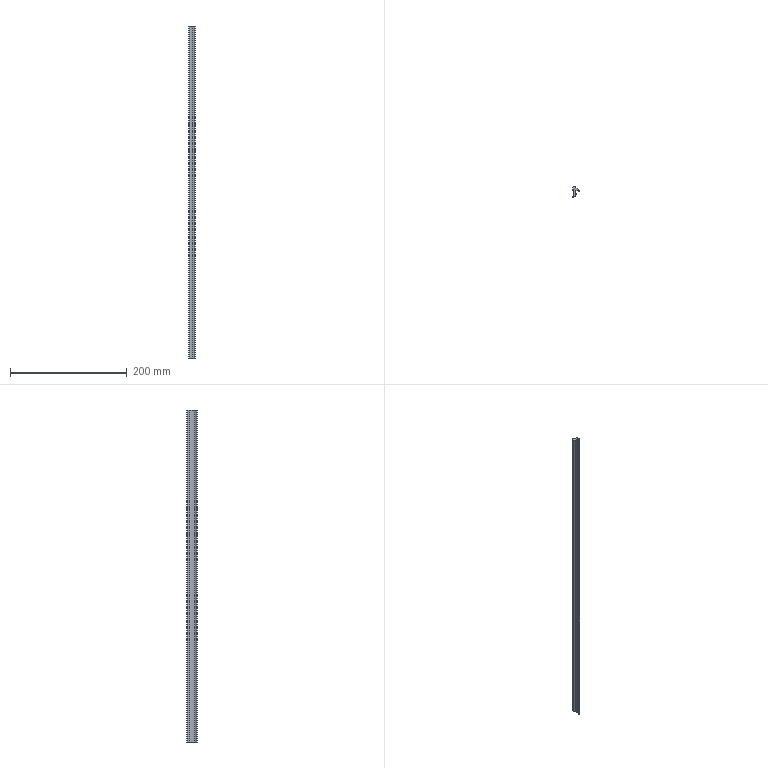Part | SolidWorks | features BaseBody 1, MoveFace 1 | 1 solid | 20 faces | box 10.8 x 17.5 x 568 mm | volume 44759 mm3 | cylinder 11 | plane 9 | commonest cylinder face diameters 1.6 x2 14 x2 0.4 x1 0.6 x1 0.8 x1 2.6 x1
STEP:
#1=CARTESIAN_POINT('',(-3.236,-11.055,468.));
#2=VERTEX_POINT('',#1);
#3=CARTESIAN_POINT('',(-4.3,-10.3,468.));
#4=VERTEX_POINT('',#3);
#5=CARTESIAN_POINT('',(-3.5,-10.3,468.));
#6=DIRECTION('',(0.,0.,-1.));
#7=DIRECTION('',(1.,0.,0.));
#8=AXIS2_PLACEMENT_3D('',#5,#6,#7);
#9=CIRCLE('',#8,0.8);
#10=EDGE_CURVE('',#2,#4,#9,.T.);
#11=ORIENTED_EDGE('',*,*,#10,.T.);
#12=CARTESIAN_POINT('',(-4.3,-10.3,-100.));
#13=VERTEX_POINT('',#12);
#14=CARTESIAN_POINT('',(-4.3,-10.3,-100.));
#15=DIRECTION('',(0.,0.,-1.));
#16=VECTOR('',#15,1000.);
#17=LINE('',#14,#16);
#18=EDGE_CURVE('',#4,#13,#17,.T.);
#19=ORIENTED_EDGE('',*,*,#18,.T.);
#20=CARTESIAN_POINT('',(-3.236,-11.055,-100.));
#21=VERTEX_POINT('',#20);
#22=CARTESIAN_POINT('',(-3.5,-10.3,-100.));
#23=DIRECTION('',(0.,0.,1.));
#24=DIRECTION('',(-1.,0.,0.));
#25=AXIS2_PLACEMENT_3D('',#22,#23,#24);
#26=CIRCLE('',#25,0.8);
#27=EDGE_CURVE('',#13,#21,#26,.T.);
#28=ORIENTED_EDGE('',*,*,#27,.T.);
#29=CARTESIAN_POINT('',(-3.236,-11.055,-100.));
#30=DIRECTION('',(0.,0.,-1.));
#31=VECTOR('',#30,1000.);
#32=LINE('',#29,#31);
#33=EDGE_CURVE('',#2,#21,#32,.T.);
#34=ORIENTED_EDGE('',*,*,#33,.F.);
#35=EDGE_LOOP('',(#11,#19,#28,#34));
#36=FACE_OUTER_BOUND('',#35,.T.);
#37=CARTESIAN_POINT('',(-3.5,-10.3,-100.));
#38=DIRECTION('',(0.,0.,-1.));
#39=DIRECTION('',(-1.,0.,0.));
#40=AXIS2_PLACEMENT_3D('',#37,#38,#39);
#41=CYLINDRICAL_SURFACE('',#40,0.8);
#42=ADVANCED_FACE('',(#36),#41,.T.);
#43=CARTESIAN_POINT('',(1.184,-6.397,-100.));
#44=VERTEX_POINT('',#43);
#45=CARTESIAN_POINT('',(-5.702,-4.29,-100.));
#46=DIRECTION('',(0.,0.,1.));
#47=DIRECTION('',(-1.,0.,0.));
#48=AXIS2_PLACEMENT_3D('',#45,#46,#47);
#49=CIRCLE('',#48,7.201);
#50=EDGE_CURVE('',#21,#44,#49,.T.);
#51=ORIENTED_EDGE('',*,*,#50,.T.);
#52=CARTESIAN_POINT('',(1.184,-6.397,468.));
#53=VERTEX_POINT('',#52);
#54=CARTESIAN_POINT('',(1.184,-6.397,-100.));
#55=DIRECTION('',(0.,0.,1.));
#56=VECTOR('',#55,1000.);
#57=LINE('',#54,#56);
#58=EDGE_CURVE('',#44,#53,#57,.T.);
#59=ORIENTED_EDGE('',*,*,#58,.T.);
#60=CARTESIAN_POINT('',(-5.702,-4.29,468.));
#61=DIRECTION('',(0.,0.,-1.));
#62=DIRECTION('',(1.,0.,0.));
#63=AXIS2_PLACEMENT_3D('',#60,#61,#62);
#64=CIRCLE('',#63,7.201);
#65=EDGE_CURVE('',#53,#2,#64,.T.);
#66=ORIENTED_EDGE('',*,*,#65,.T.);
#67=ORIENTED_EDGE('',*,*,#33,.T.);
#68=EDGE_LOOP('',(#51,#59,#66,#67));
#69=FACE_OUTER_BOUND('',#68,.T.);
#70=CARTESIAN_POINT('',(-5.702,-4.29,-100.));
#71=DIRECTION('',(0.,0.,-1.));
#72=DIRECTION('',(-1.,0.,0.));
#73=AXIS2_PLACEMENT_3D('',#70,#71,#72);
#74=CYLINDRICAL_SURFACE('',#73,7.201);
#75=ADVANCED_FACE('',(#69),#74,.T.);
#76=CARTESIAN_POINT('',(0.9,-6.,-100.));
#77=VERTEX_POINT('',#76);
#78=CARTESIAN_POINT('',(0.9,-6.3,-100.));
#79=DIRECTION('',(0.,0.,1.));
#80=DIRECTION('',(-1.,0.,0.));
#81=AXIS2_PLACEMENT_3D('',#78,#79,#80);
#82=CIRCLE('',#81,0.3);
#83=EDGE_CURVE('',#44,#77,#82,.T.);
#84=ORIENTED_EDGE('',*,*,#83,.T.);
#85=CARTESIAN_POINT('',(0.9,-6.,468.));
#86=VERTEX_POINT('',#85);
#87=CARTESIAN_POINT('',(0.9,-6.,-100.));
#88=DIRECTION('',(0.,0.,1.));
#89=VECTOR('',#88,1000.);
#90=LINE('',#87,#89);
#91=EDGE_CURVE('',#77,#86,#90,.T.);
#92=ORIENTED_EDGE('',*,*,#91,.T.);
#93=CARTESIAN_POINT('',(0.9,-6.3,468.));
#94=DIRECTION('',(0.,0.,-1.));
#95=DIRECTION('',(1.,0.,0.));
#96=AXIS2_PLACEMENT_3D('',#93,#94,#95);
#97=CIRCLE('',#96,0.3);
#98=EDGE_CURVE('',#86,#53,#97,.T.);
#99=ORIENTED_EDGE('',*,*,#98,.T.);
#100=ORIENTED_EDGE('',*,*,#58,.F.);
#101=EDGE_LOOP('',(#84,#92,#99,#100));
#102=FACE_OUTER_BOUND('',#101,.T.);
#103=CARTESIAN_POINT('',(0.9,-6.3,-100.));
#104=DIRECTION('',(0.,0.,-1.));
#105=DIRECTION('',(-1.,0.,0.));
#106=AXIS2_PLACEMENT_3D('',#103,#104,#105);
#107=CYLINDRICAL_SURFACE('',#106,0.3);
#108=ADVANCED_FACE('',(#102),#107,.T.);
#109=CARTESIAN_POINT('',(-2.5,-0.5,-100.));
#110=VERTEX_POINT('',#109);
#111=CARTESIAN_POINT('',(-2.5,-6.153,-100.));
#112=VERTEX_POINT('',#111);
#113=CARTESIAN_POINT('',(-2.5,-6.397,-100.));
#114=DIRECTION('',(0.,-1.,0.));
#115=VECTOR('',#114,1000.);
#116=LINE('',#113,#115);
#117=EDGE_CURVE('',#110,#112,#116,.T.);
#118=ORIENTED_EDGE('',*,*,#117,.F.);
#119=CARTESIAN_POINT('',(-4.2,1.695,-100.));
#120=VERTEX_POINT('',#119);
#121=CARTESIAN_POINT('',(-1.701,1.875,-100.));
#122=DIRECTION('',(0.,0.,1.));
#123=DIRECTION('',(-1.,0.,0.));
#124=AXIS2_PLACEMENT_3D('',#121,#122,#123);
#125=CIRCLE('',#124,2.506);
#126=EDGE_CURVE('',#120,#110,#125,.T.);
#127=ORIENTED_EDGE('',*,*,#126,.F.);
#128=CARTESIAN_POINT('',(-4.2,5.1,-100.));
#129=VERTEX_POINT('',#128);
#130=CARTESIAN_POINT('',(-4.2,-6.397,-100.));
#131=DIRECTION('',(0.,-1.,0.));
#132=VECTOR('',#131,1000.);
#133=LINE('',#130,#132);
#134=EDGE_CURVE('',#129,#120,#133,.T.);
#135=ORIENTED_EDGE('',*,*,#134,.F.);
#136=CARTESIAN_POINT('',(-2.892,6.4,-100.));
#137=VERTEX_POINT('',#136);
#138=CARTESIAN_POINT('',(-2.9,5.1,-100.));
#139=DIRECTION('',(0.,0.,1.));
#140=DIRECTION('',(-1.,0.,0.));
#141=AXIS2_PLACEMENT_3D('',#138,#139,#140);
#142=CIRCLE('',#141,1.3);
#143=EDGE_CURVE('',#137,#129,#142,.T.);
#144=ORIENTED_EDGE('',*,*,#143,.F.);
#145=CARTESIAN_POINT('',(0.5,5.5,-100.));
#146=VERTEX_POINT('',#145);
#147=CARTESIAN_POINT('',(-2.934,-0.5999,-100.));
#148=DIRECTION('',(0.,0.,1.));
#149=DIRECTION('',(-1.,0.,0.));
#150=AXIS2_PLACEMENT_3D('',#147,#148,#149);
#151=CIRCLE('',#150,7.);
#152=EDGE_CURVE('',#146,#137,#151,.T.);
#153=ORIENTED_EDGE('',*,*,#152,.F.);
#154=CARTESIAN_POINT('',(5.5,1.7,-100.));
#155=VERTEX_POINT('',#154);
#156=CARTESIAN_POINT('',(5.5,1.7,-100.));
#157=DIRECTION('',(-0.7962,0.6051,0.));
#158=VECTOR('',#157,1000.);
#159=LINE('',#156,#158);
#160=EDGE_CURVE('',#155,#146,#159,.T.);
#161=ORIENTED_EDGE('',*,*,#160,.F.);
#162=CARTESIAN_POINT('',(6.458,-0.2215,-100.));
#163=VERTEX_POINT('',#162);
#164=CARTESIAN_POINT('',(6.458,-0.2215,-100.));
#165=DIRECTION('',(-0.4462,0.8949,0.));
#166=VECTOR('',#165,1000.);
#167=LINE('',#164,#166);
#168=EDGE_CURVE('',#163,#155,#167,.T.);
#169=ORIENTED_EDGE('',*,*,#168,.F.);
#170=CARTESIAN_POINT('',(5.895,-0.7433,-100.));
#171=VERTEX_POINT('',#170);
#172=CARTESIAN_POINT('',(6.1,-0.4,-100.));
#173=DIRECTION('',(0.,0.,1.));
#174=DIRECTION('',(-1.,0.,0.));
#175=AXIS2_PLACEMENT_3D('',#172,#173,#174);
#176=CIRCLE('',#175,0.4);
#177=EDGE_CURVE('',#171,#163,#176,.T.);
#178=ORIENTED_EDGE('',*,*,#177,.F.);
#179=CARTESIAN_POINT('',(3.,0.,-100.));
#180=VERTEX_POINT('',#179);
#181=CARTESIAN_POINT('',(2.746,-6.995,-100.));
#182=DIRECTION('',(0.,0.,-1.));
#183=DIRECTION('',(-1.,0.,0.));
#184=AXIS2_PLACEMENT_3D('',#181,#182,#183);
#185=CIRCLE('',#184,7.);
#186=EDGE_CURVE('',#180,#171,#185,.T.);
#187=ORIENTED_EDGE('',*,*,#186,.F.);
#188=CARTESIAN_POINT('',(0.,0.,-100.));
#189=VERTEX_POINT('',#188);
#190=CARTESIAN_POINT('',(-6.814,0.,-100.));
#191=DIRECTION('',(1.,0.,0.));
#192=VECTOR('',#191,1000.);
#193=LINE('',#190,#192);
#194=EDGE_CURVE('',#189,#180,#193,.T.);
#195=ORIENTED_EDGE('',*,*,#194,.F.);
#196=CARTESIAN_POINT('',(0.,-5.8,-100.));
#197=VERTEX_POINT('',#196);
#198=CARTESIAN_POINT('',(0.,-6.397,-100.));
#199=DIRECTION('',(0.,1.,0.));
#200=VECTOR('',#199,1000.);
#201=LINE('',#198,#200);
#202=EDGE_CURVE('',#197,#189,#201,.T.);
#203=ORIENTED_EDGE('',*,*,#202,.F.);
#204=CARTESIAN_POINT('',(0.2,-6.,-100.));
#205=VERTEX_POINT('',#204);
#206=CARTESIAN_POINT('',(0.2,-5.8,-100.));
#207=DIRECTION('',(0.,0.,1.));
#208=DIRECTION('',(-1.,0.,0.));
#209=AXIS2_PLACEMENT_3D('',#206,#207,#208);
#210=CIRCLE('',#209,0.2);
#211=EDGE_CURVE('',#197,#205,#210,.T.);
#212=ORIENTED_EDGE('',*,*,#211,.T.);
#213=CARTESIAN_POINT('',(-6.814,-6.,-100.));
#214=DIRECTION('',(-1.,0.,0.));
#215=VECTOR('',#214,1000.);
#216=LINE('',#213,#215);
#217=EDGE_CURVE('',#77,#205,#216,.T.);
#218=ORIENTED_EDGE('',*,*,#217,.F.);
#219=ORIENTED_EDGE('',*,*,#83,.F.);
#220=ORIENTED_EDGE('',*,*,#50,.F.);
#221=ORIENTED_EDGE('',*,*,#27,.F.);
#222=CARTESIAN_POINT('',(-3.998,-9.674,-100.));
#223=VERTEX_POINT('',#222);
#224=CARTESIAN_POINT('',(-3.5,-10.3,-100.));
#225=DIRECTION('',(0.,0.,1.));
#226=DIRECTION('',(-1.,0.,0.));
#227=AXIS2_PLACEMENT_3D('',#224,#225,#226);
#228=CIRCLE('',#227,0.8);
#229=EDGE_CURVE('',#223,#13,#228,.T.);
#230=ORIENTED_EDGE('',*,*,#229,.F.);
#231=CARTESIAN_POINT('',(-6.814,-6.397,-100.));
#232=DIRECTION('',(0.,0.,-1.));
#233=DIRECTION('',(-1.,0.,0.));
#234=AXIS2_PLACEMENT_3D('',#231,#232,#233);
#235=CIRCLE('',#234,4.321);
#236=EDGE_CURVE('',#112,#223,#235,.T.);
#237=ORIENTED_EDGE('',*,*,#236,.F.);
#238=EDGE_LOOP('',(#118,#127,#135,#144,#153,#161,#169,#178,#187,#195,#203,#212,#218,#219,#220,#221,#230,#237));
#239=FACE_OUTER_BOUND('',#238,.T.);
#240=CARTESIAN_POINT('',(-6.814,-6.397,-100.));
#241=DIRECTION('',(0.,0.,1.));
#242=DIRECTION('',(1.,0.,0.));
#243=AXIS2_PLACEMENT_3D('',#240,#241,#242);
#244=PLANE('',#243);
#245=ADVANCED_FACE('',(#239),#244,.F.);
#246=ORIENTED_EDGE('',*,*,#18,.F.);
#247=CARTESIAN_POINT('',(-3.998,-9.674,468.));
#248=VERTEX_POINT('',#247);
#249=CARTESIAN_POINT('',(-3.5,-10.3,468.));
#250=DIRECTION('',(0.,0.,-1.));
#251=DIRECTION('',(1.,0.,0.));
#252=AXIS2_PLACEMENT_3D('',#249,#250,#251);
#253=CIRCLE('',#252,0.8);
#254=EDGE_CURVE('',#4,#248,#253,.T.);
#255=ORIENTED_EDGE('',*,*,#254,.T.);
#256=CARTESIAN_POINT('',(-3.998,-9.674,-100.));
#257=DIRECTION('',(0.,0.,-1.));
#258=VECTOR('',#257,1000.);
#259=LINE('',#256,#258);
#260=EDGE_CURVE('',#248,#223,#259,.T.);
#261=ORIENTED_EDGE('',*,*,#260,.T.);
#262=ORIENTED_EDGE('',*,*,#229,.T.);
#263=EDGE_LOOP('',(#246,#255,#261,#262));
#264=FACE_OUTER_BOUND('',#263,.T.);
#265=CARTESIAN_POINT('',(-3.5,-10.3,-100.));
#266=DIRECTION('',(0.,0.,-1.));
#267=DIRECTION('',(-1.,0.,0.));
#268=AXIS2_PLACEMENT_3D('',#265,#266,#267);
#269=CYLINDRICAL_SURFACE('',#268,0.8);
#270=ADVANCED_FACE('',(#264),#269,.T.);
#271=CARTESIAN_POINT('',(-4.2,1.695,468.));
#272=VERTEX_POINT('',#271);
#273=CARTESIAN_POINT('',(-2.5,-0.5,468.));
#274=VERTEX_POINT('',#273);
#275=CARTESIAN_POINT('',(-1.701,1.875,468.));
#276=DIRECTION('',(0.,0.,1.));
#277=DIRECTION('',(1.,0.,0.));
#278=AXIS2_PLACEMENT_3D('',#275,#276,#277);
#279=CIRCLE('',#278,2.506);
#280=EDGE_CURVE('',#272,#274,#279,.T.);
#281=ORIENTED_EDGE('',*,*,#280,.T.);
#282=CARTESIAN_POINT('',(-2.5,-6.153,468.));
#283=VERTEX_POINT('',#282);
#284=CARTESIAN_POINT('',(-2.5,-6.397,468.));
#285=DIRECTION('',(0.,-1.,0.));
#286=VECTOR('',#285,1000.);
#287=LINE('',#284,#286);
#288=EDGE_CURVE('',#274,#283,#287,.T.);
#289=ORIENTED_EDGE('',*,*,#288,.T.);
#290=CARTESIAN_POINT('',(-6.814,-6.397,468.));
#291=DIRECTION('',(0.,0.,-1.));
#292=DIRECTION('',(1.,0.,0.));
#293=AXIS2_PLACEMENT_3D('',#290,#291,#292);
#294=CIRCLE('',#293,4.321);
#295=EDGE_CURVE('',#283,#248,#294,.T.);
#296=ORIENTED_EDGE('',*,*,#295,.T.);
#297=ORIENTED_EDGE('',*,*,#254,.F.);
#298=ORIENTED_EDGE('',*,*,#10,.F.);
#299=ORIENTED_EDGE('',*,*,#65,.F.);
#300=ORIENTED_EDGE('',*,*,#98,.F.);
#301=CARTESIAN_POINT('',(0.2,-6.,468.));
#302=VERTEX_POINT('',#301);
#303=CARTESIAN_POINT('',(-6.814,-6.,468.));
#304=DIRECTION('',(-1.,0.,0.));
#305=VECTOR('',#304,1000.);
#306=LINE('',#303,#305);
#307=EDGE_CURVE('',#86,#302,#306,.T.);
#308=ORIENTED_EDGE('',*,*,#307,.T.);
#309=CARTESIAN_POINT('',(0.,-5.8,468.));
#310=VERTEX_POINT('',#309);
#311=CARTESIAN_POINT('',(0.2,-5.8,468.));
#312=DIRECTION('',(0.,0.,-1.));
#313=DIRECTION('',(1.,0.,0.));
#314=AXIS2_PLACEMENT_3D('',#311,#312,#313);
#315=CIRCLE('',#314,0.2);
#316=EDGE_CURVE('',#302,#310,#315,.T.);
#317=ORIENTED_EDGE('',*,*,#316,.T.);
#318=CARTESIAN_POINT('',(0.,0.,468.));
#319=VERTEX_POINT('',#318);
#320=CARTESIAN_POINT('',(0.,-6.397,468.));
#321=DIRECTION('',(0.,1.,0.));
#322=VECTOR('',#321,1000.);
#323=LINE('',#320,#322);
#324=EDGE_CURVE('',#310,#319,#323,.T.);
#325=ORIENTED_EDGE('',*,*,#324,.T.);
#326=CARTESIAN_POINT('',(3.,0.,468.));
#327=VERTEX_POINT('',#326);
#328=CARTESIAN_POINT('',(-6.814,0.,468.));
#329=DIRECTION('',(1.,0.,0.));
#330=VECTOR('',#329,1000.);
#331=LINE('',#328,#330);
#332=EDGE_CURVE('',#319,#327,#331,.T.);
#333=ORIENTED_EDGE('',*,*,#332,.T.);
#334=CARTESIAN_POINT('',(5.895,-0.7433,468.));
#335=VERTEX_POINT('',#334);
#336=CARTESIAN_POINT('',(2.746,-6.995,468.));
#337=DIRECTION('',(0.,0.,-1.));
#338=DIRECTION('',(1.,0.,0.));
#339=AXIS2_PLACEMENT_3D('',#336,#337,#338);
#340=CIRCLE('',#339,7.);
#341=EDGE_CURVE('',#327,#335,#340,.T.);
#342=ORIENTED_EDGE('',*,*,#341,.T.);
#343=CARTESIAN_POINT('',(6.458,-0.2215,468.));
#344=VERTEX_POINT('',#343);
#345=CARTESIAN_POINT('',(6.1,-0.4,468.));
#346=DIRECTION('',(0.,0.,-1.));
#347=DIRECTION('',(1.,0.,0.));
#348=AXIS2_PLACEMENT_3D('',#345,#346,#347);
#349=CIRCLE('',#348,0.4);
#350=EDGE_CURVE('',#344,#335,#349,.T.);
#351=ORIENTED_EDGE('',*,*,#350,.F.);
#352=CARTESIAN_POINT('',(5.5,1.7,468.));
#353=VERTEX_POINT('',#352);
#354=CARTESIAN_POINT('',(6.282,0.1323,468.));
#355=DIRECTION('',(-0.4462,0.8949,0.));
#356=VECTOR('',#355,1000.);
#357=LINE('',#354,#356);
#358=EDGE_CURVE('',#344,#353,#357,.T.);
#359=ORIENTED_EDGE('',*,*,#358,.T.);
#360=CARTESIAN_POINT('',(0.5,5.5,468.));
#361=VERTEX_POINT('',#360);
#362=CARTESIAN_POINT('',(1.595,4.668,468.));
#363=DIRECTION('',(-0.7962,0.6051,0.));
#364=VECTOR('',#363,1000.);
#365=LINE('',#362,#364);
#366=EDGE_CURVE('',#353,#361,#365,.T.);
#367=ORIENTED_EDGE('',*,*,#366,.T.);
#368=CARTESIAN_POINT('',(-2.892,6.4,468.));
#369=VERTEX_POINT('',#368);
#370=CARTESIAN_POINT('',(-2.934,-0.5999,468.));
#371=DIRECTION('',(0.,0.,1.));
#372=DIRECTION('',(1.,0.,0.));
#373=AXIS2_PLACEMENT_3D('',#370,#371,#372);
#374=CIRCLE('',#373,7.);
#375=EDGE_CURVE('',#361,#369,#374,.T.);
#376=ORIENTED_EDGE('',*,*,#375,.T.);
#377=CARTESIAN_POINT('',(-4.2,5.1,468.));
#378=VERTEX_POINT('',#377);
#379=CARTESIAN_POINT('',(-2.9,5.1,468.));
#380=DIRECTION('',(0.,0.,1.));
#381=DIRECTION('',(1.,0.,0.));
#382=AXIS2_PLACEMENT_3D('',#379,#380,#381);
#383=CIRCLE('',#382,1.3);
#384=EDGE_CURVE('',#369,#378,#383,.T.);
#385=ORIENTED_EDGE('',*,*,#384,.T.);
#386=CARTESIAN_POINT('',(-4.2,-6.397,468.));
#387=DIRECTION('',(0.,-1.,0.));
#388=VECTOR('',#387,1000.);
#389=LINE('',#386,#388);
#390=EDGE_CURVE('',#378,#272,#389,.T.);
#391=ORIENTED_EDGE('',*,*,#390,.T.);
#392=EDGE_LOOP('',(#281,#289,#296,#297,#298,#299,#300,#308,#317,#325,#333,#342,#351,#359,#367,#376,#385,#391));
#393=FACE_OUTER_BOUND('',#392,.T.);
#394=CARTESIAN_POINT('',(-6.814,-6.397,468.));
#395=DIRECTION('',(0.,0.,1.));
#396=DIRECTION('',(1.,0.,0.));
#397=AXIS2_PLACEMENT_3D('',#394,#395,#396);
#398=PLANE('',#397);
#399=ADVANCED_FACE('',(#393),#398,.T.);
#400=ORIENTED_EDGE('',*,*,#217,.T.);
#401=CARTESIAN_POINT('',(0.2,-6.,-100.));
#402=DIRECTION('',(0.,0.,1.));
#403=VECTOR('',#402,1000.);
#404=LINE('',#401,#403);
#405=EDGE_CURVE('',#205,#302,#404,.T.);
#406=ORIENTED_EDGE('',*,*,#405,.T.);
#407=ORIENTED_EDGE('',*,*,#307,.F.);
#408=ORIENTED_EDGE('',*,*,#91,.F.);
#409=EDGE_LOOP('',(#400,#406,#407,#408));
#410=FACE_OUTER_BOUND('',#409,.T.);
#411=CARTESIAN_POINT('',(0.9,-6.,-100.));
#412=DIRECTION('',(0.,1.,0.));
#413=DIRECTION('',(0.,0.,1.));
#414=AXIS2_PLACEMENT_3D('',#411,#412,#413);
#415=PLANE('',#414);
#416=ADVANCED_FACE('',(#410),#415,.T.);
#417=CARTESIAN_POINT('',(-2.5,-6.153,-100.));
#418=DIRECTION('',(0.,0.,1.));
#419=VECTOR('',#418,1000.);
#420=LINE('',#417,#419);
#421=EDGE_CURVE('',#112,#283,#420,.T.);
#422=ORIENTED_EDGE('',*,*,#421,.F.);
#423=ORIENTED_EDGE('',*,*,#236,.T.);
#424=ORIENTED_EDGE('',*,*,#260,.F.);
#425=ORIENTED_EDGE('',*,*,#295,.F.);
#426=EDGE_LOOP('',(#422,#423,#424,#425));
#427=FACE_OUTER_BOUND('',#426,.T.);
#428=CARTESIAN_POINT('',(-6.814,-6.397,-100.));
#429=DIRECTION('',(0.,0.,-1.));
#430=DIRECTION('',(-1.,0.,0.));
#431=AXIS2_PLACEMENT_3D('',#428,#429,#430);
#432=CYLINDRICAL_SURFACE('',#431,4.321);
#433=ADVANCED_FACE('',(#427),#432,.F.);
#434=ORIENTED_EDGE('',*,*,#117,.T.);
#435=ORIENTED_EDGE('',*,*,#421,.T.);
#436=ORIENTED_EDGE('',*,*,#288,.F.);
#437=CARTESIAN_POINT('',(-2.5,-0.5,-100.));
#438=DIRECTION('',(0.,0.,-1.));
#439=VECTOR('',#438,1000.);
#440=LINE('',#437,#439);
#441=EDGE_CURVE('',#274,#110,#440,.T.);
#442=ORIENTED_EDGE('',*,*,#441,.T.);
#443=EDGE_LOOP('',(#434,#435,#436,#442));
#444=FACE_OUTER_BOUND('',#443,.T.);
#445=CARTESIAN_POINT('',(-2.5,-0.5,-100.));
#446=DIRECTION('',(-1.,0.,0.));
#447=DIRECTION('',(0.,0.,1.));
#448=AXIS2_PLACEMENT_3D('',#445,#446,#447);
#449=PLANE('',#448);
#450=ADVANCED_FACE('',(#444),#449,.T.);
#451=ORIENTED_EDGE('',*,*,#126,.T.);
#452=ORIENTED_EDGE('',*,*,#441,.F.);
#453=ORIENTED_EDGE('',*,*,#280,.F.);
#454=CARTESIAN_POINT('',(-4.2,1.695,-100.));
#455=DIRECTION('',(0.,0.,-1.));
#456=VECTOR('',#455,1000.);
#457=LINE('',#454,#456);
#458=EDGE_CURVE('',#272,#120,#457,.T.);
#459=ORIENTED_EDGE('',*,*,#458,.T.);
#460=EDGE_LOOP('',(#451,#452,#453,#459));
#461=FACE_OUTER_BOUND('',#460,.T.);
#462=CARTESIAN_POINT('',(-1.701,1.875,-100.));
#463=DIRECTION('',(0.,0.,-1.));
#464=DIRECTION('',(-1.,0.,0.));
#465=AXIS2_PLACEMENT_3D('',#462,#463,#464);
#466=CYLINDRICAL_SURFACE('',#465,2.506);
#467=ADVANCED_FACE('',(#461),#466,.T.);
#468=ORIENTED_EDGE('',*,*,#134,.T.);
#469=ORIENTED_EDGE('',*,*,#458,.F.);
#470=ORIENTED_EDGE('',*,*,#390,.F.);
#471=CARTESIAN_POINT('',(-4.2,5.1,-100.));
#472=DIRECTION('',(0.,0.,-1.));
#473=VECTOR('',#472,1000.);
#474=LINE('',#471,#473);
#475=EDGE_CURVE('',#378,#129,#474,.T.);
#476=ORIENTED_EDGE('',*,*,#475,.T.);
#477=EDGE_LOOP('',(#468,#469,#470,#476));
#478=FACE_OUTER_BOUND('',#477,.T.);
#479=CARTESIAN_POINT('',(-4.2,5.1,-100.));
#480=DIRECTION('',(-1.,0.,0.));
#481=DIRECTION('',(0.,0.,1.));
#482=AXIS2_PLACEMENT_3D('',#479,#480,#481);
#483=PLANE('',#482);
#484=ADVANCED_FACE('',(#478),#483,.T.);
#485=ORIENTED_EDGE('',*,*,#143,.T.);
#486=ORIENTED_EDGE('',*,*,#475,.F.);
#487=ORIENTED_EDGE('',*,*,#384,.F.);
#488=CARTESIAN_POINT('',(-2.892,6.4,-100.));
#489=DIRECTION('',(0.,0.,-1.));
#490=VECTOR('',#489,1000.);
#491=LINE('',#488,#490);
#492=EDGE_CURVE('',#369,#137,#491,.T.);
#493=ORIENTED_EDGE('',*,*,#492,.T.);
#494=EDGE_LOOP('',(#485,#486,#487,#493));
#495=FACE_OUTER_BOUND('',#494,.T.);
#496=CARTESIAN_POINT('',(-2.9,5.1,-100.));
#497=DIRECTION('',(0.,0.,-1.));
#498=DIRECTION('',(-1.,0.,0.));
#499=AXIS2_PLACEMENT_3D('',#496,#497,#498);
#500=CYLINDRICAL_SURFACE('',#499,1.3);
#501=ADVANCED_FACE('',(#495),#500,.T.);
#502=ORIENTED_EDGE('',*,*,#152,.T.);
#503=ORIENTED_EDGE('',*,*,#492,.F.);
#504=ORIENTED_EDGE('',*,*,#375,.F.);
#505=CARTESIAN_POINT('',(0.5,5.5,-100.));
#506=DIRECTION('',(0.,0.,-1.));
#507=VECTOR('',#506,1000.);
#508=LINE('',#505,#507);
#509=EDGE_CURVE('',#361,#146,#508,.T.);
#510=ORIENTED_EDGE('',*,*,#509,.T.);
#511=EDGE_LOOP('',(#502,#503,#504,#510));
#512=FACE_OUTER_BOUND('',#511,.T.);
#513=CARTESIAN_POINT('',(-2.934,-0.5999,-100.));
#514=DIRECTION('',(0.,0.,-1.));
#515=DIRECTION('',(-1.,0.,0.));
#516=AXIS2_PLACEMENT_3D('',#513,#514,#515);
#517=CYLINDRICAL_SURFACE('',#516,7.);
#518=ADVANCED_FACE('',(#512),#517,.T.);
#519=ORIENTED_EDGE('',*,*,#160,.T.);
#520=ORIENTED_EDGE('',*,*,#509,.F.);
#521=ORIENTED_EDGE('',*,*,#366,.F.);
#522=CARTESIAN_POINT('',(5.5,1.7,-100.));
#523=DIRECTION('',(0.,0.,-1.));
#524=VECTOR('',#523,1000.);
#525=LINE('',#522,#524);
#526=EDGE_CURVE('',#353,#155,#525,.T.);
#527=ORIENTED_EDGE('',*,*,#526,.T.);
#528=EDGE_LOOP('',(#519,#520,#521,#527));
#529=FACE_OUTER_BOUND('',#528,.T.);
#530=CARTESIAN_POINT('',(5.5,1.7,-100.));
#531=DIRECTION('',(0.6051,0.7962,0.));
#532=DIRECTION('',(-0.7962,0.6051,0.));
#533=AXIS2_PLACEMENT_3D('',#530,#531,#532);
#534=PLANE('',#533);
#535=ADVANCED_FACE('',(#529),#534,.T.);
#536=ORIENTED_EDGE('',*,*,#168,.T.);
#537=ORIENTED_EDGE('',*,*,#526,.F.);
#538=ORIENTED_EDGE('',*,*,#358,.F.);
#539=CARTESIAN_POINT('',(6.458,-0.2215,-100.));
#540=DIRECTION('',(0.,0.,-1.));
#541=VECTOR('',#540,1000.);
#542=LINE('',#539,#541);
#543=EDGE_CURVE('',#344,#163,#542,.T.);
#544=ORIENTED_EDGE('',*,*,#543,.T.);
#545=EDGE_LOOP('',(#536,#537,#538,#544));
#546=FACE_OUTER_BOUND('',#545,.T.);
#547=CARTESIAN_POINT('',(6.458,-0.2215,-100.));
#548=DIRECTION('',(0.8949,0.4462,0.));
#549=DIRECTION('',(-0.4462,0.8949,0.));
#550=AXIS2_PLACEMENT_3D('',#547,#548,#549);
#551=PLANE('',#550);
#552=ADVANCED_FACE('',(#546),#551,.T.);
#553=CARTESIAN_POINT('',(3.,0.,-100.));
#554=DIRECTION('',(0.,0.,1.));
#555=VECTOR('',#554,1000.);
#556=LINE('',#553,#555);
#557=EDGE_CURVE('',#180,#327,#556,.T.);
#558=ORIENTED_EDGE('',*,*,#557,.F.);
#559=ORIENTED_EDGE('',*,*,#186,.T.);
#560=CARTESIAN_POINT('',(5.895,-0.7433,-100.));
#561=DIRECTION('',(0.,0.,-1.));
#562=VECTOR('',#561,1000.);
#563=LINE('',#560,#562);
#564=EDGE_CURVE('',#335,#171,#563,.T.);
#565=ORIENTED_EDGE('',*,*,#564,.F.);
#566=ORIENTED_EDGE('',*,*,#341,.F.);
#567=EDGE_LOOP('',(#558,#559,#565,#566));
#568=FACE_OUTER_BOUND('',#567,.T.);
#569=CARTESIAN_POINT('',(2.746,-6.995,-100.));
#570=DIRECTION('',(0.,0.,-1.));
#571=DIRECTION('',(-1.,0.,0.));
#572=AXIS2_PLACEMENT_3D('',#569,#570,#571);
#573=CYLINDRICAL_SURFACE('',#572,7.);
#574=ADVANCED_FACE('',(#568),#573,.F.);
#575=ORIENTED_EDGE('',*,*,#194,.T.);
#576=ORIENTED_EDGE('',*,*,#557,.T.);
#577=ORIENTED_EDGE('',*,*,#332,.F.);
#578=CARTESIAN_POINT('',(0.,0.,-100.));
#579=DIRECTION('',(0.,0.,-1.));
#580=VECTOR('',#579,1000.);
#581=LINE('',#578,#580);
#582=EDGE_CURVE('',#319,#189,#581,.T.);
#583=ORIENTED_EDGE('',*,*,#582,.T.);
#584=EDGE_LOOP('',(#575,#576,#577,#583));
#585=FACE_OUTER_BOUND('',#584,.T.);
#586=CARTESIAN_POINT('',(0.,0.,-100.));
#587=DIRECTION('',(0.,-1.,0.));
#588=DIRECTION('',(0.,0.,-1.));
#589=AXIS2_PLACEMENT_3D('',#586,#587,#588);
#590=PLANE('',#589);
#591=ADVANCED_FACE('',(#585),#590,.T.);
#592=ORIENTED_EDGE('',*,*,#202,.T.);
#593=ORIENTED_EDGE('',*,*,#582,.F.);
#594=ORIENTED_EDGE('',*,*,#324,.F.);
#595=CARTESIAN_POINT('',(0.,-5.8,-100.));
#596=DIRECTION('',(0.,0.,-1.));
#597=VECTOR('',#596,1000.);
#598=LINE('',#595,#597);
#599=EDGE_CURVE('',#310,#197,#598,.T.);
#600=ORIENTED_EDGE('',*,*,#599,.T.);
#601=EDGE_LOOP('',(#592,#593,#594,#600));
#602=FACE_OUTER_BOUND('',#601,.T.);
#603=CARTESIAN_POINT('',(0.,-5.8,-100.));
#604=DIRECTION('',(1.,0.,0.));
#605=DIRECTION('',(0.,0.,-1.));
#606=AXIS2_PLACEMENT_3D('',#603,#604,#605);
#607=PLANE('',#606);
#608=ADVANCED_FACE('',(#602),#607,.T.);
#609=ORIENTED_EDGE('',*,*,#405,.F.);
#610=ORIENTED_EDGE('',*,*,#211,.F.);
#611=ORIENTED_EDGE('',*,*,#599,.F.);
#612=ORIENTED_EDGE('',*,*,#316,.F.);
#613=EDGE_LOOP('',(#609,#610,#611,#612));
#614=FACE_OUTER_BOUND('',#613,.T.);
#615=CARTESIAN_POINT('',(0.2,-5.8,-100.));
#616=DIRECTION('',(0.,0.,-1.));
#617=DIRECTION('',(-1.,0.,0.));
#618=AXIS2_PLACEMENT_3D('',#615,#616,#617);
#619=CYLINDRICAL_SURFACE('',#618,0.2);
#620=ADVANCED_FACE('',(#614),#619,.F.);
#621=ORIENTED_EDGE('',*,*,#177,.T.);
#622=ORIENTED_EDGE('',*,*,#543,.F.);
#623=ORIENTED_EDGE('',*,*,#350,.T.);
#624=ORIENTED_EDGE('',*,*,#564,.T.);
#625=EDGE_LOOP('',(#621,#622,#623,#624));
#626=FACE_OUTER_BOUND('',#625,.T.);
#627=CARTESIAN_POINT('',(6.1,-0.4,-100.));
#628=DIRECTION('',(0.,0.,-1.));
#629=DIRECTION('',(-1.,0.,0.));
#630=AXIS2_PLACEMENT_3D('',#627,#628,#629);
#631=CYLINDRICAL_SURFACE('',#630,0.4);
#632=ADVANCED_FACE('',(#626),#631,.T.);
#633=CLOSED_SHELL('',(#42,#75,#108,#245,#270,#399,#416,#433,#450,#467,#484,#501,#518,#535,#552,#574,#591,#608,#620,#632));
#634=MANIFOLD_SOLID_BREP('',#633);
#635=CARTESIAN_POINT('',(0.,0.,0.));
#636=DIRECTION('',(0.,0.,1.));
#637=DIRECTION('',(1.,0.,0.));
#638=AXIS2_PLACEMENT_3D('',#635,#636,#637);
#639=(LENGTH_UNIT()NAMED_UNIT(*)SI_UNIT(.MILLI.,.METRE.));
#640=UNCERTAINTY_MEASURE_WITH_UNIT(LENGTH_MEASURE(0.00001),#639,'','');
#641=(NAMED_UNIT(*)PLANE_ANGLE_UNIT()SI_UNIT($,.RADIAN.));
#642=(NAMED_UNIT(*)SI_UNIT($,.STERADIAN.)SOLID_ANGLE_UNIT());
#643=(GEOMETRIC_REPRESENTATION_CONTEXT(3)GLOBAL_UNCERTAINTY_ASSIGNED_CONTEXT((#640))GLOBAL_UNIT_ASSIGNED_CONTEXT((#639,#641,#642))REPRESENTATION_CONTEXT('',''));
#644=ADVANCED_BREP_SHAPE_REPRESENTATION('',(#634,#638),#643);